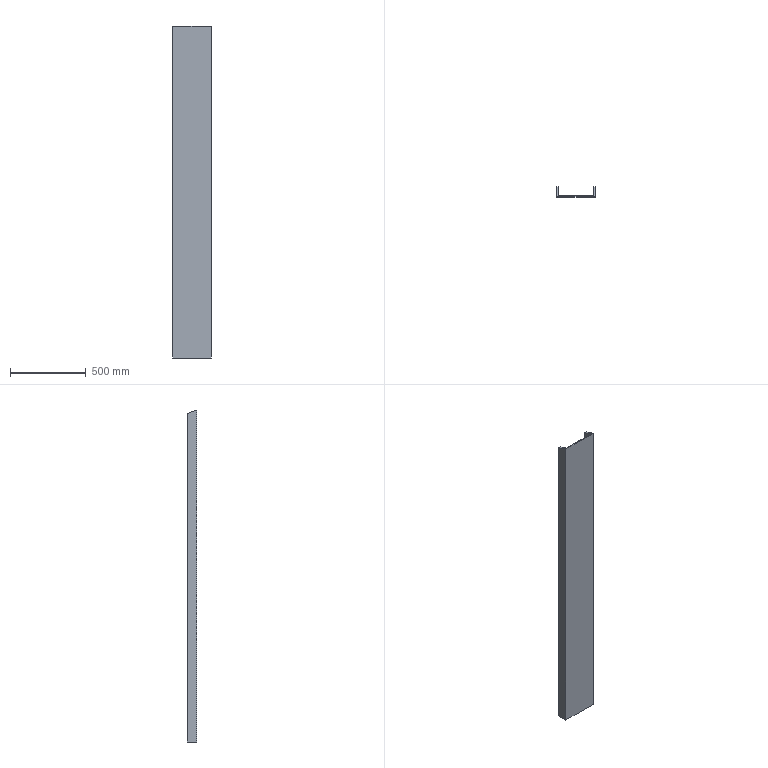Part | SolidWorks | features Extrusion 1, ICE 1 | 1 solid | 10 faces | box 254 x 66.04 x 2199 mm | volume 6305556 mm3 | plane 10
STEP:
#1=CARTESIAN_POINT('',(127.,66.04,1076.753));
#2=VERTEX_POINT('',#1);
#3=CARTESIAN_POINT('',(127.,66.04,-1099.338));
#4=VERTEX_POINT('',#3);
#5=CARTESIAN_POINT('',(127.,66.04,1099.338));
#6=DIRECTION('',(0.,0.,-1.));
#7=VECTOR('',#6,1000.);
#8=LINE('',#5,#7);
#9=EDGE_CURVE('',#2,#4,#8,.T.);
#10=ORIENTED_EDGE('',*,*,#9,.F.);
#11=CARTESIAN_POINT('',(127.,0.,1099.338));
#12=VERTEX_POINT('',#11);
#13=CARTESIAN_POINT('',(127.,59.125,1079.118));
#14=DIRECTION('',(0.,-0.9462,0.3236));
#15=VECTOR('',#14,1000.);
#16=LINE('',#13,#15);
#17=EDGE_CURVE('',#2,#12,#16,.T.);
#18=ORIENTED_EDGE('',*,*,#17,.T.);
#19=CARTESIAN_POINT('',(127.,0.,-1099.338));
#20=VERTEX_POINT('',#19);
#21=CARTESIAN_POINT('',(127.,0.,1099.338));
#22=DIRECTION('',(0.,0.,-1.));
#23=VECTOR('',#22,1000.);
#24=LINE('',#21,#23);
#25=EDGE_CURVE('',#12,#20,#24,.T.);
#26=ORIENTED_EDGE('',*,*,#25,.T.);
#27=CARTESIAN_POINT('',(127.,66.04,-1099.338));
#28=DIRECTION('',(0.,1.,0.));
#29=VECTOR('',#28,1000.);
#30=LINE('',#27,#29);
#31=EDGE_CURVE('',#20,#4,#30,.T.);
#32=ORIENTED_EDGE('',*,*,#31,.T.);
#33=EDGE_LOOP('',(#10,#18,#26,#32));
#34=FACE_OUTER_BOUND('',#33,.T.);
#35=CARTESIAN_POINT('',(127.,66.04,1099.338));
#36=DIRECTION('',(-1.,0.,0.));
#37=DIRECTION('',(0.,0.,1.));
#38=AXIS2_PLACEMENT_3D('',#35,#36,#37);
#39=PLANE('',#38);
#40=ADVANCED_FACE('',(#34),#39,.F.);
#41=CARTESIAN_POINT('',(115.926,66.04,1076.753));
#42=VERTEX_POINT('',#41);
#43=CARTESIAN_POINT('',(115.926,66.04,-1099.338));
#44=VERTEX_POINT('',#43);
#45=CARTESIAN_POINT('',(115.926,66.04,1099.338));
#46=DIRECTION('',(0.,0.,-1.));
#47=VECTOR('',#46,1000.);
#48=LINE('',#45,#47);
#49=EDGE_CURVE('',#42,#44,#48,.T.);
#50=ORIENTED_EDGE('',*,*,#49,.F.);
#51=CARTESIAN_POINT('',(-150.,66.04,1076.753));
#52=DIRECTION('',(1.,0.,0.));
#53=VECTOR('',#52,1000.);
#54=LINE('',#51,#53);
#55=EDGE_CURVE('',#42,#2,#54,.T.);
#56=ORIENTED_EDGE('',*,*,#55,.T.);
#57=ORIENTED_EDGE('',*,*,#9,.T.);
#58=CARTESIAN_POINT('',(115.926,66.04,-1099.338));
#59=DIRECTION('',(-1.,0.,0.));
#60=VECTOR('',#59,1000.);
#61=LINE('',#58,#60);
#62=EDGE_CURVE('',#4,#44,#61,.T.);
#63=ORIENTED_EDGE('',*,*,#62,.T.);
#64=EDGE_LOOP('',(#50,#56,#57,#63));
#65=FACE_OUTER_BOUND('',#64,.T.);
#66=CARTESIAN_POINT('',(115.926,66.04,1099.338));
#67=DIRECTION('',(0.,-1.,0.));
#68=DIRECTION('',(0.,0.,-1.));
#69=AXIS2_PLACEMENT_3D('',#66,#67,#68);
#70=PLANE('',#69);
#71=ADVANCED_FACE('',(#65),#70,.F.);
#72=CARTESIAN_POINT('',(115.926,6.096,1097.253));
#73=VERTEX_POINT('',#72);
#74=CARTESIAN_POINT('',(115.926,6.096,-1099.338));
#75=VERTEX_POINT('',#74);
#76=CARTESIAN_POINT('',(115.926,6.096,1099.338));
#77=DIRECTION('',(0.,0.,-1.));
#78=VECTOR('',#77,1000.);
#79=LINE('',#76,#78);
#80=EDGE_CURVE('',#73,#75,#79,.T.);
#81=ORIENTED_EDGE('',*,*,#80,.F.);
#82=CARTESIAN_POINT('',(115.926,5.458,1097.471));
#83=DIRECTION('',(0.,0.9462,-0.3236));
#84=VECTOR('',#83,1000.);
#85=LINE('',#82,#84);
#86=EDGE_CURVE('',#73,#42,#85,.T.);
#87=ORIENTED_EDGE('',*,*,#86,.T.);
#88=ORIENTED_EDGE('',*,*,#49,.T.);
#89=CARTESIAN_POINT('',(115.926,6.096,-1099.338));
#90=DIRECTION('',(0.,-1.,0.));
#91=VECTOR('',#90,1000.);
#92=LINE('',#89,#91);
#93=EDGE_CURVE('',#44,#75,#92,.T.);
#94=ORIENTED_EDGE('',*,*,#93,.T.);
#95=EDGE_LOOP('',(#81,#87,#88,#94));
#96=FACE_OUTER_BOUND('',#95,.T.);
#97=CARTESIAN_POINT('',(115.926,6.096,1099.338));
#98=DIRECTION('',(1.,0.,0.));
#99=DIRECTION('',(0.,0.,-1.));
#100=AXIS2_PLACEMENT_3D('',#97,#98,#99);
#101=PLANE('',#100);
#102=ADVANCED_FACE('',(#96),#101,.F.);
#103=CARTESIAN_POINT('',(-115.926,6.096,1097.253));
#104=VERTEX_POINT('',#103);
#105=CARTESIAN_POINT('',(-115.926,6.096,-1099.338));
#106=VERTEX_POINT('',#105);
#107=CARTESIAN_POINT('',(-115.926,6.096,1099.338));
#108=DIRECTION('',(0.,0.,-1.));
#109=VECTOR('',#108,1000.);
#110=LINE('',#107,#109);
#111=EDGE_CURVE('',#104,#106,#110,.T.);
#112=ORIENTED_EDGE('',*,*,#111,.F.);
#113=CARTESIAN_POINT('',(-115.926,6.096,1097.253));
#114=DIRECTION('',(1.,0.,0.));
#115=VECTOR('',#114,1000.);
#116=LINE('',#113,#115);
#117=EDGE_CURVE('',#104,#73,#116,.T.);
#118=ORIENTED_EDGE('',*,*,#117,.T.);
#119=ORIENTED_EDGE('',*,*,#80,.T.);
#120=CARTESIAN_POINT('',(-115.926,6.096,-1099.338));
#121=DIRECTION('',(-1.,0.,0.));
#122=VECTOR('',#121,1000.);
#123=LINE('',#120,#122);
#124=EDGE_CURVE('',#75,#106,#123,.T.);
#125=ORIENTED_EDGE('',*,*,#124,.T.);
#126=EDGE_LOOP('',(#112,#118,#119,#125));
#127=FACE_OUTER_BOUND('',#126,.T.);
#128=CARTESIAN_POINT('',(-115.926,6.096,1099.338));
#129=DIRECTION('',(0.,-1.,0.));
#130=DIRECTION('',(0.,0.,-1.));
#131=AXIS2_PLACEMENT_3D('',#128,#129,#130);
#132=PLANE('',#131);
#133=ADVANCED_FACE('',(#127),#132,.F.);
#134=CARTESIAN_POINT('',(-115.926,66.04,1076.753));
#135=VERTEX_POINT('',#134);
#136=CARTESIAN_POINT('',(-115.926,66.04,-1099.338));
#137=VERTEX_POINT('',#136);
#138=CARTESIAN_POINT('',(-115.926,66.04,1099.338));
#139=DIRECTION('',(0.,0.,-1.));
#140=VECTOR('',#139,1000.);
#141=LINE('',#138,#140);
#142=EDGE_CURVE('',#135,#137,#141,.T.);
#143=ORIENTED_EDGE('',*,*,#142,.F.);
#144=CARTESIAN_POINT('',(-115.926,59.125,1079.118));
#145=DIRECTION('',(0.,-0.9462,0.3236));
#146=VECTOR('',#145,1000.);
#147=LINE('',#144,#146);
#148=EDGE_CURVE('',#135,#104,#147,.T.);
#149=ORIENTED_EDGE('',*,*,#148,.T.);
#150=ORIENTED_EDGE('',*,*,#111,.T.);
#151=CARTESIAN_POINT('',(-115.926,66.04,-1099.338));
#152=DIRECTION('',(0.,1.,0.));
#153=VECTOR('',#152,1000.);
#154=LINE('',#151,#153);
#155=EDGE_CURVE('',#106,#137,#154,.T.);
#156=ORIENTED_EDGE('',*,*,#155,.T.);
#157=EDGE_LOOP('',(#143,#149,#150,#156));
#158=FACE_OUTER_BOUND('',#157,.T.);
#159=CARTESIAN_POINT('',(-115.926,66.04,1099.338));
#160=DIRECTION('',(-1.,0.,0.));
#161=DIRECTION('',(0.,-1.,0.));
#162=AXIS2_PLACEMENT_3D('',#159,#160,#161);
#163=PLANE('',#162);
#164=ADVANCED_FACE('',(#158),#163,.F.);
#165=CARTESIAN_POINT('',(-127.,66.04,1076.753));
#166=VERTEX_POINT('',#165);
#167=CARTESIAN_POINT('',(-127.,66.04,-1099.338));
#168=VERTEX_POINT('',#167);
#169=CARTESIAN_POINT('',(-127.,66.04,1099.338));
#170=DIRECTION('',(0.,0.,-1.));
#171=VECTOR('',#170,1000.);
#172=LINE('',#169,#171);
#173=EDGE_CURVE('',#166,#168,#172,.T.);
#174=ORIENTED_EDGE('',*,*,#173,.F.);
#175=CARTESIAN_POINT('',(-150.,66.04,1076.753));
#176=DIRECTION('',(1.,0.,0.));
#177=VECTOR('',#176,1000.);
#178=LINE('',#175,#177);
#179=EDGE_CURVE('',#166,#135,#178,.T.);
#180=ORIENTED_EDGE('',*,*,#179,.T.);
#181=ORIENTED_EDGE('',*,*,#142,.T.);
#182=CARTESIAN_POINT('',(-127.,66.04,-1099.338));
#183=DIRECTION('',(-1.,0.,0.));
#184=VECTOR('',#183,1000.);
#185=LINE('',#182,#184);
#186=EDGE_CURVE('',#137,#168,#185,.T.);
#187=ORIENTED_EDGE('',*,*,#186,.T.);
#188=EDGE_LOOP('',(#174,#180,#181,#187));
#189=FACE_OUTER_BOUND('',#188,.T.);
#190=CARTESIAN_POINT('',(-127.,66.04,1099.338));
#191=DIRECTION('',(0.,-1.,0.));
#192=DIRECTION('',(0.,0.,-1.));
#193=AXIS2_PLACEMENT_3D('',#190,#191,#192);
#194=PLANE('',#193);
#195=ADVANCED_FACE('',(#189),#194,.F.);
#196=CARTESIAN_POINT('',(-127.,0.,1099.338));
#197=VERTEX_POINT('',#196);
#198=CARTESIAN_POINT('',(-127.,0.,-1099.338));
#199=VERTEX_POINT('',#198);
#200=CARTESIAN_POINT('',(-127.,0.,1099.338));
#201=DIRECTION('',(0.,0.,-1.));
#202=VECTOR('',#201,1000.);
#203=LINE('',#200,#202);
#204=EDGE_CURVE('',#197,#199,#203,.T.);
#205=ORIENTED_EDGE('',*,*,#204,.F.);
#206=CARTESIAN_POINT('',(-127.,0.,1099.338));
#207=DIRECTION('',(0.,0.9462,-0.3236));
#208=VECTOR('',#207,1000.);
#209=LINE('',#206,#208);
#210=EDGE_CURVE('',#197,#166,#209,.T.);
#211=ORIENTED_EDGE('',*,*,#210,.T.);
#212=ORIENTED_EDGE('',*,*,#173,.T.);
#213=CARTESIAN_POINT('',(-127.,0.,-1099.338));
#214=DIRECTION('',(0.,-1.,0.));
#215=VECTOR('',#214,1000.);
#216=LINE('',#213,#215);
#217=EDGE_CURVE('',#168,#199,#216,.T.);
#218=ORIENTED_EDGE('',*,*,#217,.T.);
#219=EDGE_LOOP('',(#205,#211,#212,#218));
#220=FACE_OUTER_BOUND('',#219,.T.);
#221=CARTESIAN_POINT('',(-127.,0.,1099.338));
#222=DIRECTION('',(1.,0.,0.));
#223=DIRECTION('',(0.,0.,-1.));
#224=AXIS2_PLACEMENT_3D('',#221,#222,#223);
#225=PLANE('',#224);
#226=ADVANCED_FACE('',(#220),#225,.F.);
#227=CARTESIAN_POINT('',(127.,0.,-1099.338));
#228=DIRECTION('',(1.,0.,0.));
#229=VECTOR('',#228,1000.);
#230=LINE('',#227,#229);
#231=EDGE_CURVE('',#199,#20,#230,.T.);
#232=ORIENTED_EDGE('',*,*,#231,.T.);
#233=ORIENTED_EDGE('',*,*,#25,.F.);
#234=CARTESIAN_POINT('',(127.,0.,1099.338));
#235=DIRECTION('',(1.,0.,0.));
#236=VECTOR('',#235,1000.);
#237=LINE('',#234,#236);
#238=EDGE_CURVE('',#197,#12,#237,.T.);
#239=ORIENTED_EDGE('',*,*,#238,.F.);
#240=ORIENTED_EDGE('',*,*,#204,.T.);
#241=EDGE_LOOP('',(#232,#233,#239,#240));
#242=FACE_OUTER_BOUND('',#241,.T.);
#243=CARTESIAN_POINT('',(127.,0.,1099.338));
#244=DIRECTION('',(0.,1.,0.));
#245=DIRECTION('',(0.,0.,1.));
#246=AXIS2_PLACEMENT_3D('',#243,#244,#245);
#247=PLANE('',#246);
#248=ADVANCED_FACE('',(#242),#247,.F.);
#249=ORIENTED_EDGE('',*,*,#31,.F.);
#250=ORIENTED_EDGE('',*,*,#231,.F.);
#251=ORIENTED_EDGE('',*,*,#217,.F.);
#252=ORIENTED_EDGE('',*,*,#186,.F.);
#253=ORIENTED_EDGE('',*,*,#155,.F.);
#254=ORIENTED_EDGE('',*,*,#124,.F.);
#255=ORIENTED_EDGE('',*,*,#93,.F.);
#256=ORIENTED_EDGE('',*,*,#62,.F.);
#257=EDGE_LOOP('',(#249,#250,#251,#252,#253,#254,#255,#256));
#258=FACE_OUTER_BOUND('',#257,.T.);
#259=CARTESIAN_POINT('',(127.,0.,-1099.338));
#260=DIRECTION('',(0.,0.,-1.));
#261=DIRECTION('',(-1.,0.,0.));
#262=AXIS2_PLACEMENT_3D('',#259,#260,#261);
#263=PLANE('',#262);
#264=ADVANCED_FACE('',(#258),#263,.T.);
#265=ORIENTED_EDGE('',*,*,#55,.F.);
#266=ORIENTED_EDGE('',*,*,#86,.F.);
#267=ORIENTED_EDGE('',*,*,#117,.F.);
#268=ORIENTED_EDGE('',*,*,#148,.F.);
#269=ORIENTED_EDGE('',*,*,#179,.F.);
#270=ORIENTED_EDGE('',*,*,#210,.F.);
#271=ORIENTED_EDGE('',*,*,#238,.T.);
#272=ORIENTED_EDGE('',*,*,#17,.F.);
#273=EDGE_LOOP('',(#265,#266,#267,#268,#269,#270,#271,#272));
#274=FACE_OUTER_BOUND('',#273,.T.);
#275=CARTESIAN_POINT('',(-150.,0.,1099.338));
#276=DIRECTION('',(0.,-0.3236,-0.9462));
#277=DIRECTION('',(0.,0.9462,-0.3236));
#278=AXIS2_PLACEMENT_3D('',#275,#276,#277);
#279=PLANE('',#278);
#280=ADVANCED_FACE('',(#274),#279,.F.);
#281=CLOSED_SHELL('',(#40,#71,#102,#133,#164,#195,#226,#248,#264,#280));
#282=MANIFOLD_SOLID_BREP('',#281);
#283=CARTESIAN_POINT('',(0.,0.,0.));
#284=DIRECTION('',(0.,0.,1.));
#285=DIRECTION('',(1.,0.,0.));
#286=AXIS2_PLACEMENT_3D('',#283,#284,#285);
#287=(LENGTH_UNIT()NAMED_UNIT(*)SI_UNIT(.MILLI.,.METRE.));
#288=UNCERTAINTY_MEASURE_WITH_UNIT(LENGTH_MEASURE(0.00001),#287,'','');
#289=(NAMED_UNIT(*)PLANE_ANGLE_UNIT()SI_UNIT($,.RADIAN.));
#290=(NAMED_UNIT(*)SI_UNIT($,.STERADIAN.)SOLID_ANGLE_UNIT());
#291=(GEOMETRIC_REPRESENTATION_CONTEXT(3)GLOBAL_UNCERTAINTY_ASSIGNED_CONTEXT((#288))GLOBAL_UNIT_ASSIGNED_CONTEXT((#287,#289,#290))REPRESENTATION_CONTEXT('',''));
#292=ADVANCED_BREP_SHAPE_REPRESENTATION('',(#282,#286),#291);